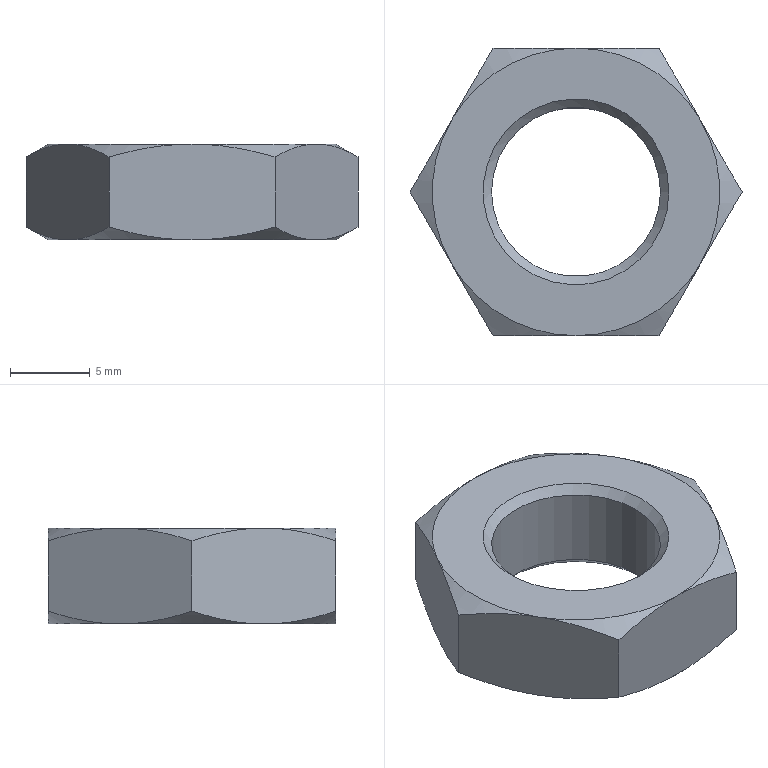Part | NX | features META 3, SKETCH 3, DATUM_CSYS 2, EXTRUDE 2, SWP104 2, CHAMFER 1, LINE 1, SYMBOLIC_THREAD 1, THREADS 1 | 1 solid | 23 faces | box 20.785 x 18 x 6 mm | volume 1134 mm3 | cone 14 | plane 8 | cylinder 1 | commonest cylinder face diameters 10.579 x1
STEP:
#1=CARTESIAN_POINT('',(5.819,0.,6.));
#2=VERTEX_POINT('',#1);
#3=CARTESIAN_POINT('',(0.,0.,6.));
#4=DIRECTION('',(0.,0.,1.));
#5=DIRECTION('',(1.,0.,0.));
#6=AXIS2_PLACEMENT_3D('',#3,#4,#5);
#7=CIRCLE('',#6,5.819);
#8=EDGE_CURVE('',#2,#2,#7,.F.);
#9=ORIENTED_EDGE('',*,*,#8,.T.);
#10=EDGE_LOOP('',(#9));
#11=FACE_BOUND('',#10,.T.);
#12=CARTESIAN_POINT('',(-7.794,4.5,6.));
#13=VERTEX_POINT('',#12);
#14=CARTESIAN_POINT('',(0.,9.,6.));
#15=VERTEX_POINT('',#14);
#16=CARTESIAN_POINT('',(0.,0.,6.));
#17=DIRECTION('',(0.,0.,-1.));
#18=DIRECTION('',(-1.,0.,0.));
#19=AXIS2_PLACEMENT_3D('',#16,#17,#18);
#20=CIRCLE('',#19,9.);
#21=EDGE_CURVE('',#13,#15,#20,.T.);
#22=ORIENTED_EDGE('',*,*,#21,.F.);
#23=CARTESIAN_POINT('',(-7.794,-4.5,6.));
#24=VERTEX_POINT('',#23);
#25=CARTESIAN_POINT('',(0.,0.,6.));
#26=DIRECTION('',(0.,0.,-1.));
#27=DIRECTION('',(-1.,0.,0.));
#28=AXIS2_PLACEMENT_3D('',#25,#26,#27);
#29=CIRCLE('',#28,9.);
#30=EDGE_CURVE('',#24,#13,#29,.T.);
#31=ORIENTED_EDGE('',*,*,#30,.F.);
#32=CARTESIAN_POINT('',(0.,-9.,6.));
#33=VERTEX_POINT('',#32);
#34=CARTESIAN_POINT('',(0.,0.,6.));
#35=DIRECTION('',(0.,0.,-1.));
#36=DIRECTION('',(-1.,0.,0.));
#37=AXIS2_PLACEMENT_3D('',#34,#35,#36);
#38=CIRCLE('',#37,9.);
#39=EDGE_CURVE('',#33,#24,#38,.T.);
#40=ORIENTED_EDGE('',*,*,#39,.F.);
#41=CARTESIAN_POINT('',(7.794,-4.5,6.));
#42=VERTEX_POINT('',#41);
#43=CARTESIAN_POINT('',(0.,0.,6.));
#44=DIRECTION('',(0.,0.,-1.));
#45=DIRECTION('',(-1.,0.,0.));
#46=AXIS2_PLACEMENT_3D('',#43,#44,#45);
#47=CIRCLE('',#46,9.);
#48=EDGE_CURVE('',#42,#33,#47,.T.);
#49=ORIENTED_EDGE('',*,*,#48,.F.);
#50=CARTESIAN_POINT('',(7.794,4.5,6.));
#51=VERTEX_POINT('',#50);
#52=CARTESIAN_POINT('',(0.,0.,6.));
#53=DIRECTION('',(0.,0.,-1.));
#54=DIRECTION('',(-1.,0.,0.));
#55=AXIS2_PLACEMENT_3D('',#52,#53,#54);
#56=CIRCLE('',#55,9.);
#57=EDGE_CURVE('',#51,#42,#56,.T.);
#58=ORIENTED_EDGE('',*,*,#57,.F.);
#59=CARTESIAN_POINT('',(0.,0.,6.));
#60=DIRECTION('',(0.,0.,-1.));
#61=DIRECTION('',(-1.,0.,0.));
#62=AXIS2_PLACEMENT_3D('',#59,#60,#61);
#63=CIRCLE('',#62,9.);
#64=EDGE_CURVE('',#15,#51,#63,.T.);
#65=ORIENTED_EDGE('',*,*,#64,.F.);
#66=EDGE_LOOP('',(#22,#31,#40,#49,#58,#65));
#67=FACE_BOUND('',#66,.T.);
#68=CARTESIAN_POINT('',(0.,18.,6.));
#69=DIRECTION('',(0.,0.,1.));
#70=DIRECTION('',(1.,0.,0.));
#71=AXIS2_PLACEMENT_3D('',#68,#69,#70);
#72=PLANE('',#71);
#73=ADVANCED_FACE('',(#11,#67),#72,.T.);
#74=CARTESIAN_POINT('',(5.819,0.,0.));
#75=VERTEX_POINT('',#74);
#76=CARTESIAN_POINT('',(0.,0.,0.));
#77=DIRECTION('',(0.,0.,1.));
#78=DIRECTION('',(1.,0.,0.));
#79=AXIS2_PLACEMENT_3D('',#76,#77,#78);
#80=CIRCLE('',#79,5.819);
#81=EDGE_CURVE('',#75,#75,#80,.T.);
#82=ORIENTED_EDGE('',*,*,#81,.T.);
#83=EDGE_LOOP('',(#82));
#84=FACE_BOUND('',#83,.T.);
#85=CARTESIAN_POINT('',(-7.794,-4.5,0.));
#86=VERTEX_POINT('',#85);
#87=CARTESIAN_POINT('',(-7.794,4.5,0.));
#88=VERTEX_POINT('',#87);
#89=CARTESIAN_POINT('',(0.,0.,0.));
#90=DIRECTION('',(0.,0.,-1.));
#91=DIRECTION('',(-1.,0.,0.));
#92=AXIS2_PLACEMENT_3D('',#89,#90,#91);
#93=CIRCLE('',#92,9.);
#94=EDGE_CURVE('',#86,#88,#93,.T.);
#95=ORIENTED_EDGE('',*,*,#94,.T.);
#96=CARTESIAN_POINT('',(0.,9.,0.));
#97=VERTEX_POINT('',#96);
#98=CARTESIAN_POINT('',(0.,0.,0.));
#99=DIRECTION('',(0.,0.,-1.));
#100=DIRECTION('',(-1.,0.,0.));
#101=AXIS2_PLACEMENT_3D('',#98,#99,#100);
#102=CIRCLE('',#101,9.);
#103=EDGE_CURVE('',#88,#97,#102,.T.);
#104=ORIENTED_EDGE('',*,*,#103,.T.);
#105=CARTESIAN_POINT('',(7.794,4.5,0.));
#106=VERTEX_POINT('',#105);
#107=CARTESIAN_POINT('',(0.,0.,0.));
#108=DIRECTION('',(0.,0.,-1.));
#109=DIRECTION('',(-1.,0.,0.));
#110=AXIS2_PLACEMENT_3D('',#107,#108,#109);
#111=CIRCLE('',#110,9.);
#112=EDGE_CURVE('',#97,#106,#111,.T.);
#113=ORIENTED_EDGE('',*,*,#112,.T.);
#114=CARTESIAN_POINT('',(7.794,-4.5,0.));
#115=VERTEX_POINT('',#114);
#116=CARTESIAN_POINT('',(0.,0.,0.));
#117=DIRECTION('',(0.,0.,-1.));
#118=DIRECTION('',(-1.,0.,0.));
#119=AXIS2_PLACEMENT_3D('',#116,#117,#118);
#120=CIRCLE('',#119,9.);
#121=EDGE_CURVE('',#106,#115,#120,.T.);
#122=ORIENTED_EDGE('',*,*,#121,.T.);
#123=CARTESIAN_POINT('',(0.,-9.,0.));
#124=VERTEX_POINT('',#123);
#125=CARTESIAN_POINT('',(0.,0.,0.));
#126=DIRECTION('',(0.,0.,-1.));
#127=DIRECTION('',(-1.,0.,0.));
#128=AXIS2_PLACEMENT_3D('',#125,#126,#127);
#129=CIRCLE('',#128,9.);
#130=EDGE_CURVE('',#115,#124,#129,.T.);
#131=ORIENTED_EDGE('',*,*,#130,.T.);
#132=CARTESIAN_POINT('',(0.,0.,0.));
#133=DIRECTION('',(0.,0.,-1.));
#134=DIRECTION('',(-1.,0.,0.));
#135=AXIS2_PLACEMENT_3D('',#132,#133,#134);
#136=CIRCLE('',#135,9.);
#137=EDGE_CURVE('',#124,#86,#136,.T.);
#138=ORIENTED_EDGE('',*,*,#137,.T.);
#139=EDGE_LOOP('',(#95,#104,#113,#122,#131,#138));
#140=FACE_BOUND('',#139,.T.);
#141=CARTESIAN_POINT('',(0.,18.,0.));
#142=DIRECTION('',(0.,0.,1.));
#143=DIRECTION('',(1.,0.,0.));
#144=AXIS2_PLACEMENT_3D('',#141,#142,#143);
#145=PLANE('',#144);
#146=ADVANCED_FACE('',(#84,#140),#145,.F.);
#147=CARTESIAN_POINT('',(10.392,0.,5.196));
#148=VERTEX_POINT('',#147);
#149=CARTESIAN_POINT('',(10.392,0.,0.8038));
#150=VERTEX_POINT('',#149);
#151=CARTESIAN_POINT('',(10.392,0.,6.));
#152=DIRECTION('',(0.,0.,-1.));
#153=VECTOR('',#152,1000.);
#154=LINE('',#151,#153);
#155=EDGE_CURVE('',#148,#150,#154,.T.);
#156=ORIENTED_EDGE('',*,*,#155,.T.);
#157=CARTESIAN_POINT('',(10.392,0.,0.8038));
#158=CARTESIAN_POINT('',(9.542,1.472,0.3131));
#159=CARTESIAN_POINT('',(8.679,2.967,0.));
#160=CARTESIAN_POINT('',(7.794,4.5,0.));
#161=B_SPLINE_CURVE_WITH_KNOTS('',3,(#157,#158,#159,#160),.UNSPECIFIED.,.F.,.F.,(4,4),(0.000000238,0.005258),.UNSPECIFIED.);
#162=EDGE_CURVE('',#150,#106,#161,.T.);
#163=ORIENTED_EDGE('',*,*,#162,.T.);
#164=CARTESIAN_POINT('',(5.196,9.,0.8038));
#165=VERTEX_POINT('',#164);
#166=CARTESIAN_POINT('',(7.794,4.5,0.));
#167=CARTESIAN_POINT('',(6.912,6.028,0.));
#168=CARTESIAN_POINT('',(6.044,7.531,0.3143));
#169=CARTESIAN_POINT('',(5.196,9.,0.8038));
#170=B_SPLINE_CURVE_WITH_KNOTS('',3,(#166,#167,#168,#169),.UNSPECIFIED.,.F.,.F.,(4,4),(0.005258,0.0105),.UNSPECIFIED.);
#171=EDGE_CURVE('',#106,#165,#170,.T.);
#172=ORIENTED_EDGE('',*,*,#171,.T.);
#173=CARTESIAN_POINT('',(5.196,9.,5.196));
#174=VERTEX_POINT('',#173);
#175=CARTESIAN_POINT('',(5.196,9.,6.));
#176=DIRECTION('',(0.,0.,-1.));
#177=VECTOR('',#176,1000.);
#178=LINE('',#175,#177);
#179=EDGE_CURVE('',#174,#165,#178,.T.);
#180=ORIENTED_EDGE('',*,*,#179,.F.);
#181=CARTESIAN_POINT('',(5.196,9.,5.196));
#182=CARTESIAN_POINT('',(6.046,7.528,5.687));
#183=CARTESIAN_POINT('',(6.909,6.033,6.));
#184=CARTESIAN_POINT('',(7.794,4.5,6.));
#185=B_SPLINE_CURVE_WITH_KNOTS('',3,(#181,#182,#183,#184),.UNSPECIFIED.,.F.,.F.,(4,4),(0.000000238,0.005258),.UNSPECIFIED.);
#186=EDGE_CURVE('',#174,#51,#185,.T.);
#187=ORIENTED_EDGE('',*,*,#186,.T.);
#188=CARTESIAN_POINT('',(7.794,4.5,6.));
#189=CARTESIAN_POINT('',(8.676,2.972,6.));
#190=CARTESIAN_POINT('',(9.544,1.469,5.686));
#191=CARTESIAN_POINT('',(10.392,0.,5.196));
#192=B_SPLINE_CURVE_WITH_KNOTS('',3,(#188,#189,#190,#191),.UNSPECIFIED.,.F.,.F.,(4,4),(0.005258,0.0105),.UNSPECIFIED.);
#193=EDGE_CURVE('',#51,#148,#192,.T.);
#194=ORIENTED_EDGE('',*,*,#193,.T.);
#195=EDGE_LOOP('',(#156,#163,#172,#180,#187,#194));
#196=FACE_BOUND('',#195,.T.);
#197=CARTESIAN_POINT('',(5.196,9.,6.));
#198=DIRECTION('',(0.866,0.5,0.));
#199=DIRECTION('',(-0.5,0.866,0.));
#200=AXIS2_PLACEMENT_3D('',#197,#198,#199);
#201=PLANE('',#200);
#202=ADVANCED_FACE('',(#196),#201,.T.);
#203=CARTESIAN_POINT('',(5.196,-9.,5.196));
#204=VERTEX_POINT('',#203);
#205=CARTESIAN_POINT('',(5.196,-9.,0.8038));
#206=VERTEX_POINT('',#205);
#207=CARTESIAN_POINT('',(5.196,-9.,6.));
#208=DIRECTION('',(0.,0.,-1.));
#209=VECTOR('',#208,1000.);
#210=LINE('',#207,#209);
#211=EDGE_CURVE('',#204,#206,#210,.T.);
#212=ORIENTED_EDGE('',*,*,#211,.T.);
#213=CARTESIAN_POINT('',(5.196,-9.,0.8038));
#214=CARTESIAN_POINT('',(6.046,-7.528,0.3131));
#215=CARTESIAN_POINT('',(6.909,-6.033,0.));
#216=CARTESIAN_POINT('',(7.794,-4.5,0.));
#217=B_SPLINE_CURVE_WITH_KNOTS('',3,(#213,#214,#215,#216),.UNSPECIFIED.,.F.,.F.,(4,4),(0.000000238,0.005258),.UNSPECIFIED.);
#218=EDGE_CURVE('',#206,#115,#217,.T.);
#219=ORIENTED_EDGE('',*,*,#218,.T.);
#220=CARTESIAN_POINT('',(7.794,-4.5,0.));
#221=CARTESIAN_POINT('',(8.676,-2.972,0.));
#222=CARTESIAN_POINT('',(9.544,-1.469,0.3143));
#223=CARTESIAN_POINT('',(10.392,0.,0.8038));
#224=B_SPLINE_CURVE_WITH_KNOTS('',3,(#220,#221,#222,#223),.UNSPECIFIED.,.F.,.F.,(4,4),(0.005258,0.0105),.UNSPECIFIED.);
#225=EDGE_CURVE('',#115,#150,#224,.T.);
#226=ORIENTED_EDGE('',*,*,#225,.T.);
#227=ORIENTED_EDGE('',*,*,#155,.F.);
#228=CARTESIAN_POINT('',(10.392,0.,5.196));
#229=CARTESIAN_POINT('',(9.542,-1.472,5.687));
#230=CARTESIAN_POINT('',(8.679,-2.967,6.));
#231=CARTESIAN_POINT('',(7.794,-4.5,6.));
#232=B_SPLINE_CURVE_WITH_KNOTS('',3,(#228,#229,#230,#231),.UNSPECIFIED.,.F.,.F.,(4,4),(0.000000238,0.005258),.UNSPECIFIED.);
#233=EDGE_CURVE('',#148,#42,#232,.T.);
#234=ORIENTED_EDGE('',*,*,#233,.T.);
#235=CARTESIAN_POINT('',(7.794,-4.5,6.));
#236=CARTESIAN_POINT('',(6.912,-6.028,6.));
#237=CARTESIAN_POINT('',(6.044,-7.531,5.686));
#238=CARTESIAN_POINT('',(5.196,-9.,5.196));
#239=B_SPLINE_CURVE_WITH_KNOTS('',3,(#235,#236,#237,#238),.UNSPECIFIED.,.F.,.F.,(4,4),(0.005258,0.0105),.UNSPECIFIED.);
#240=EDGE_CURVE('',#42,#204,#239,.T.);
#241=ORIENTED_EDGE('',*,*,#240,.T.);
#242=EDGE_LOOP('',(#212,#219,#226,#227,#234,#241));
#243=FACE_BOUND('',#242,.T.);
#244=CARTESIAN_POINT('',(10.392,0.,6.));
#245=DIRECTION('',(0.866,-0.5,0.));
#246=DIRECTION('',(0.5,0.866,0.));
#247=AXIS2_PLACEMENT_3D('',#244,#245,#246);
#248=PLANE('',#247);
#249=ADVANCED_FACE('',(#243),#248,.T.);
#250=CARTESIAN_POINT('',(-5.196,-9.,5.196));
#251=VERTEX_POINT('',#250);
#252=CARTESIAN_POINT('',(-5.196,-9.,0.8038));
#253=VERTEX_POINT('',#252);
#254=CARTESIAN_POINT('',(-5.196,-9.,6.));
#255=DIRECTION('',(0.,0.,-1.));
#256=VECTOR('',#255,1000.);
#257=LINE('',#254,#256);
#258=EDGE_CURVE('',#251,#253,#257,.T.);
#259=ORIENTED_EDGE('',*,*,#258,.T.);
#260=CARTESIAN_POINT('',(-5.196,-9.,0.8038));
#261=CARTESIAN_POINT('',(-3.506,-9.,0.3159));
#262=CARTESIAN_POINT('',(-1.756,-9.,0.));
#263=CARTESIAN_POINT('',(0.,-9.,0.));
#264=B_SPLINE_CURVE_WITH_KNOTS('',3,(#260,#261,#262,#263),.UNSPECIFIED.,.F.,.F.,(4,4),(0.009271,0.01453),.UNSPECIFIED.);
#265=EDGE_CURVE('',#253,#124,#264,.T.);
#266=ORIENTED_EDGE('',*,*,#265,.T.);
#267=CARTESIAN_POINT('',(0.,-9.,0.));
#268=CARTESIAN_POINT('',(1.757,-9.,0.));
#269=CARTESIAN_POINT('',(3.516,-9.,0.3188));
#270=CARTESIAN_POINT('',(5.196,-9.,0.8038));
#271=B_SPLINE_CURVE_WITH_KNOTS('',3,(#267,#268,#269,#270),.UNSPECIFIED.,.F.,.F.,(4,4),(0.01453,0.01979),.UNSPECIFIED.);
#272=EDGE_CURVE('',#124,#206,#271,.T.);
#273=ORIENTED_EDGE('',*,*,#272,.T.);
#274=ORIENTED_EDGE('',*,*,#211,.F.);
#275=CARTESIAN_POINT('',(0.,-9.,6.));
#276=CARTESIAN_POINT('',(1.757,-9.,6.));
#277=CARTESIAN_POINT('',(3.516,-9.,5.681));
#278=CARTESIAN_POINT('',(5.196,-9.,5.196));
#279=B_SPLINE_CURVE_WITH_KNOTS('',3,(#275,#276,#277,#278),.UNSPECIFIED.,.F.,.F.,(4,4),(0.01453,0.01979),.UNSPECIFIED.);
#280=EDGE_CURVE('',#204,#33,#279,.F.);
#281=ORIENTED_EDGE('',*,*,#280,.T.);
#282=CARTESIAN_POINT('',(-5.196,-9.,5.196));
#283=CARTESIAN_POINT('',(-3.506,-9.,5.684));
#284=CARTESIAN_POINT('',(-1.756,-9.,6.));
#285=CARTESIAN_POINT('',(0.,-9.,6.));
#286=B_SPLINE_CURVE_WITH_KNOTS('',3,(#282,#283,#284,#285),.UNSPECIFIED.,.F.,.F.,(4,4),(0.009271,0.01453),.UNSPECIFIED.);
#287=EDGE_CURVE('',#33,#251,#286,.F.);
#288=ORIENTED_EDGE('',*,*,#287,.T.);
#289=EDGE_LOOP('',(#259,#266,#273,#274,#281,#288));
#290=FACE_BOUND('',#289,.T.);
#291=CARTESIAN_POINT('',(5.196,-9.,6.));
#292=DIRECTION('',(0.,-1.,0.));
#293=DIRECTION('',(0.,0.,-1.));
#294=AXIS2_PLACEMENT_3D('',#291,#292,#293);
#295=PLANE('',#294);
#296=ADVANCED_FACE('',(#290),#295,.T.);
#297=CARTESIAN_POINT('',(-10.392,0.,5.196));
#298=VERTEX_POINT('',#297);
#299=CARTESIAN_POINT('',(-10.392,0.,0.8038));
#300=VERTEX_POINT('',#299);
#301=CARTESIAN_POINT('',(-10.392,0.,6.));
#302=DIRECTION('',(0.,0.,-1.));
#303=VECTOR('',#302,1000.);
#304=LINE('',#301,#303);
#305=EDGE_CURVE('',#298,#300,#304,.T.);
#306=ORIENTED_EDGE('',*,*,#305,.T.);
#307=CARTESIAN_POINT('',(-10.392,0.,0.8038));
#308=CARTESIAN_POINT('',(-9.542,-1.472,0.3131));
#309=CARTESIAN_POINT('',(-8.679,-2.967,0.));
#310=CARTESIAN_POINT('',(-7.794,-4.5,0.));
#311=B_SPLINE_CURVE_WITH_KNOTS('',3,(#307,#308,#309,#310),.UNSPECIFIED.,.F.,.F.,(4,4),(0.000000238,0.005258),.UNSPECIFIED.);
#312=EDGE_CURVE('',#300,#86,#311,.T.);
#313=ORIENTED_EDGE('',*,*,#312,.T.);
#314=CARTESIAN_POINT('',(-7.794,-4.5,0.));
#315=CARTESIAN_POINT('',(-6.912,-6.028,0.));
#316=CARTESIAN_POINT('',(-6.044,-7.531,0.3143));
#317=CARTESIAN_POINT('',(-5.196,-9.,0.8038));
#318=B_SPLINE_CURVE_WITH_KNOTS('',3,(#314,#315,#316,#317),.UNSPECIFIED.,.F.,.F.,(4,4),(0.005258,0.0105),.UNSPECIFIED.);
#319=EDGE_CURVE('',#86,#253,#318,.T.);
#320=ORIENTED_EDGE('',*,*,#319,.T.);
#321=ORIENTED_EDGE('',*,*,#258,.F.);
#322=CARTESIAN_POINT('',(-5.196,-9.,5.196));
#323=CARTESIAN_POINT('',(-6.046,-7.528,5.687));
#324=CARTESIAN_POINT('',(-6.909,-6.033,6.));
#325=CARTESIAN_POINT('',(-7.794,-4.5,6.));
#326=B_SPLINE_CURVE_WITH_KNOTS('',3,(#322,#323,#324,#325),.UNSPECIFIED.,.F.,.F.,(4,4),(0.000000238,0.005258),.UNSPECIFIED.);
#327=EDGE_CURVE('',#251,#24,#326,.T.);
#328=ORIENTED_EDGE('',*,*,#327,.T.);
#329=CARTESIAN_POINT('',(-7.794,-4.5,6.));
#330=CARTESIAN_POINT('',(-8.676,-2.972,6.));
#331=CARTESIAN_POINT('',(-9.544,-1.469,5.686));
#332=CARTESIAN_POINT('',(-10.392,0.,5.196));
#333=B_SPLINE_CURVE_WITH_KNOTS('',3,(#329,#330,#331,#332),.UNSPECIFIED.,.F.,.F.,(4,4),(0.005258,0.0105),.UNSPECIFIED.);
#334=EDGE_CURVE('',#24,#298,#333,.T.);
#335=ORIENTED_EDGE('',*,*,#334,.T.);
#336=EDGE_LOOP('',(#306,#313,#320,#321,#328,#335));
#337=FACE_BOUND('',#336,.T.);
#338=CARTESIAN_POINT('',(-5.196,-9.,6.));
#339=DIRECTION('',(-0.866,-0.5,0.));
#340=DIRECTION('',(0.5,-0.866,0.));
#341=AXIS2_PLACEMENT_3D('',#338,#339,#340);
#342=PLANE('',#341);
#343=ADVANCED_FACE('',(#337),#342,.T.);
#344=CARTESIAN_POINT('',(-5.196,9.,5.196));
#345=VERTEX_POINT('',#344);
#346=CARTESIAN_POINT('',(-5.196,9.,0.8038));
#347=VERTEX_POINT('',#346);
#348=CARTESIAN_POINT('',(-5.196,9.,6.));
#349=DIRECTION('',(0.,0.,-1.));
#350=VECTOR('',#349,1000.);
#351=LINE('',#348,#350);
#352=EDGE_CURVE('',#345,#347,#351,.T.);
#353=ORIENTED_EDGE('',*,*,#352,.T.);
#354=CARTESIAN_POINT('',(-5.196,9.,0.8038));
#355=CARTESIAN_POINT('',(-6.046,7.528,0.3131));
#356=CARTESIAN_POINT('',(-6.909,6.033,0.));
#357=CARTESIAN_POINT('',(-7.794,4.5,0.));
#358=B_SPLINE_CURVE_WITH_KNOTS('',3,(#354,#355,#356,#357),.UNSPECIFIED.,.F.,.F.,(4,4),(0.000000238,0.005258),.UNSPECIFIED.);
#359=EDGE_CURVE('',#347,#88,#358,.T.);
#360=ORIENTED_EDGE('',*,*,#359,.T.);
#361=CARTESIAN_POINT('',(-7.794,4.5,0.));
#362=CARTESIAN_POINT('',(-8.676,2.972,0.));
#363=CARTESIAN_POINT('',(-9.544,1.469,0.3143));
#364=CARTESIAN_POINT('',(-10.392,0.,0.8038));
#365=B_SPLINE_CURVE_WITH_KNOTS('',3,(#361,#362,#363,#364),.UNSPECIFIED.,.F.,.F.,(4,4),(0.005258,0.0105),.UNSPECIFIED.);
#366=EDGE_CURVE('',#88,#300,#365,.T.);
#367=ORIENTED_EDGE('',*,*,#366,.T.);
#368=ORIENTED_EDGE('',*,*,#305,.F.);
#369=CARTESIAN_POINT('',(-10.392,0.,5.196));
#370=CARTESIAN_POINT('',(-9.542,1.472,5.687));
#371=CARTESIAN_POINT('',(-8.679,2.967,6.));
#372=CARTESIAN_POINT('',(-7.794,4.5,6.));
#373=B_SPLINE_CURVE_WITH_KNOTS('',3,(#369,#370,#371,#372),.UNSPECIFIED.,.F.,.F.,(4,4),(0.000000238,0.005258),.UNSPECIFIED.);
#374=EDGE_CURVE('',#298,#13,#373,.T.);
#375=ORIENTED_EDGE('',*,*,#374,.T.);
#376=CARTESIAN_POINT('',(-7.794,4.5,6.));
#377=CARTESIAN_POINT('',(-6.912,6.028,6.));
#378=CARTESIAN_POINT('',(-6.044,7.531,5.686));
#379=CARTESIAN_POINT('',(-5.196,9.,5.196));
#380=B_SPLINE_CURVE_WITH_KNOTS('',3,(#376,#377,#378,#379),.UNSPECIFIED.,.F.,.F.,(4,4),(0.005258,0.0105),.UNSPECIFIED.);
#381=EDGE_CURVE('',#13,#345,#380,.T.);
#382=ORIENTED_EDGE('',*,*,#381,.T.);
#383=EDGE_LOOP('',(#353,#360,#367,#368,#375,#382));
#384=FACE_BOUND('',#383,.T.);
#385=CARTESIAN_POINT('',(-10.392,0.,6.));
#386=DIRECTION('',(-0.866,0.5,0.));
#387=DIRECTION('',(-0.5,-0.866,0.));
#388=AXIS2_PLACEMENT_3D('',#385,#386,#387);
#389=PLANE('',#388);
#390=ADVANCED_FACE('',(#384),#389,.T.);
#391=ORIENTED_EDGE('',*,*,#179,.T.);
#392=CARTESIAN_POINT('',(0.,9.,0.));
#393=CARTESIAN_POINT('',(1.757,9.,0.));
#394=CARTESIAN_POINT('',(3.516,9.,0.3188));
#395=CARTESIAN_POINT('',(5.196,9.,0.8038));
#396=B_SPLINE_CURVE_WITH_KNOTS('',3,(#392,#393,#394,#395),.UNSPECIFIED.,.F.,.F.,(4,4),(0.01453,0.01979),.UNSPECIFIED.);
#397=EDGE_CURVE('',#165,#97,#396,.F.);
#398=ORIENTED_EDGE('',*,*,#397,.T.);
#399=CARTESIAN_POINT('',(-5.196,9.,0.8038));
#400=CARTESIAN_POINT('',(-3.506,9.,0.3159));
#401=CARTESIAN_POINT('',(-1.756,9.,0.));
#402=CARTESIAN_POINT('',(0.,9.,0.));
#403=B_SPLINE_CURVE_WITH_KNOTS('',3,(#399,#400,#401,#402),.UNSPECIFIED.,.F.,.F.,(4,4),(0.009271,0.01453),.UNSPECIFIED.);
#404=EDGE_CURVE('',#97,#347,#403,.F.);
#405=ORIENTED_EDGE('',*,*,#404,.T.);
#406=ORIENTED_EDGE('',*,*,#352,.F.);
#407=CARTESIAN_POINT('',(-5.196,9.,5.196));
#408=CARTESIAN_POINT('',(-3.506,9.,5.684));
#409=CARTESIAN_POINT('',(-1.756,9.,6.));
#410=CARTESIAN_POINT('',(0.,9.,6.));
#411=B_SPLINE_CURVE_WITH_KNOTS('',3,(#407,#408,#409,#410),.UNSPECIFIED.,.F.,.F.,(4,4),(0.009271,0.01453),.UNSPECIFIED.);
#412=EDGE_CURVE('',#345,#15,#411,.T.);
#413=ORIENTED_EDGE('',*,*,#412,.T.);
#414=CARTESIAN_POINT('',(0.,9.,6.));
#415=CARTESIAN_POINT('',(1.757,9.,6.));
#416=CARTESIAN_POINT('',(3.516,9.,5.681));
#417=CARTESIAN_POINT('',(5.196,9.,5.196));
#418=B_SPLINE_CURVE_WITH_KNOTS('',3,(#414,#415,#416,#417),.UNSPECIFIED.,.F.,.F.,(4,4),(0.01453,0.01979),.UNSPECIFIED.);
#419=EDGE_CURVE('',#15,#174,#418,.T.);
#420=ORIENTED_EDGE('',*,*,#419,.T.);
#421=EDGE_LOOP('',(#391,#398,#405,#406,#413,#420));
#422=FACE_BOUND('',#421,.T.);
#423=CARTESIAN_POINT('',(-5.196,9.,6.));
#424=DIRECTION('',(0.,1.,0.));
#425=DIRECTION('',(0.,0.,1.));
#426=AXIS2_PLACEMENT_3D('',#423,#424,#425);
#427=PLANE('',#426);
#428=ADVANCED_FACE('',(#422),#427,.T.);
#429=ORIENTED_EDGE('',*,*,#419,.F.);
#430=ORIENTED_EDGE('',*,*,#64,.T.);
#431=ORIENTED_EDGE('',*,*,#186,.F.);
#432=EDGE_LOOP('',(#429,#430,#431));
#433=FACE_BOUND('',#432,.T.);
#434=CARTESIAN_POINT('',(0.,0.,5.196));
#435=DIRECTION('',(0.,0.,-1.));
#436=DIRECTION('',(-1.,0.,0.));
#437=AXIS2_PLACEMENT_3D('',#434,#435,#436);
#438=CONICAL_SURFACE('',#437,10.392,1.047);
#439=ADVANCED_FACE('',(#433),#438,.T.);
#440=ORIENTED_EDGE('',*,*,#21,.T.);
#441=ORIENTED_EDGE('',*,*,#412,.F.);
#442=ORIENTED_EDGE('',*,*,#381,.F.);
#443=EDGE_LOOP('',(#440,#441,#442));
#444=FACE_BOUND('',#443,.T.);
#445=CARTESIAN_POINT('',(0.,0.,5.196));
#446=DIRECTION('',(0.,0.,-1.));
#447=DIRECTION('',(-1.,0.,0.));
#448=AXIS2_PLACEMENT_3D('',#445,#446,#447);
#449=CONICAL_SURFACE('',#448,10.392,1.047);
#450=ADVANCED_FACE('',(#444),#449,.T.);
#451=ORIENTED_EDGE('',*,*,#30,.T.);
#452=ORIENTED_EDGE('',*,*,#374,.F.);
#453=ORIENTED_EDGE('',*,*,#334,.F.);
#454=EDGE_LOOP('',(#451,#452,#453));
#455=FACE_BOUND('',#454,.T.);
#456=CARTESIAN_POINT('',(0.,0.,5.196));
#457=DIRECTION('',(0.,0.,-1.));
#458=DIRECTION('',(-1.,0.,0.));
#459=AXIS2_PLACEMENT_3D('',#456,#457,#458);
#460=CONICAL_SURFACE('',#459,10.392,1.047);
#461=ADVANCED_FACE('',(#455),#460,.T.);
#462=ORIENTED_EDGE('',*,*,#39,.T.);
#463=ORIENTED_EDGE('',*,*,#327,.F.);
#464=ORIENTED_EDGE('',*,*,#287,.F.);
#465=EDGE_LOOP('',(#462,#463,#464));
#466=FACE_BOUND('',#465,.T.);
#467=CARTESIAN_POINT('',(0.,0.,5.196));
#468=DIRECTION('',(0.,0.,-1.));
#469=DIRECTION('',(-1.,0.,0.));
#470=AXIS2_PLACEMENT_3D('',#467,#468,#469);
#471=CONICAL_SURFACE('',#470,10.392,1.047);
#472=ADVANCED_FACE('',(#466),#471,.T.);
#473=ORIENTED_EDGE('',*,*,#48,.T.);
#474=ORIENTED_EDGE('',*,*,#280,.F.);
#475=ORIENTED_EDGE('',*,*,#240,.F.);
#476=EDGE_LOOP('',(#473,#474,#475));
#477=FACE_BOUND('',#476,.T.);
#478=CARTESIAN_POINT('',(0.,0.,5.196));
#479=DIRECTION('',(0.,0.,-1.));
#480=DIRECTION('',(-1.,0.,0.));
#481=AXIS2_PLACEMENT_3D('',#478,#479,#480);
#482=CONICAL_SURFACE('',#481,10.392,1.047);
#483=ADVANCED_FACE('',(#477),#482,.T.);
#484=ORIENTED_EDGE('',*,*,#57,.T.);
#485=ORIENTED_EDGE('',*,*,#233,.F.);
#486=ORIENTED_EDGE('',*,*,#193,.F.);
#487=EDGE_LOOP('',(#484,#485,#486));
#488=FACE_BOUND('',#487,.T.);
#489=CARTESIAN_POINT('',(0.,0.,5.196));
#490=DIRECTION('',(0.,0.,-1.));
#491=DIRECTION('',(-1.,0.,0.));
#492=AXIS2_PLACEMENT_3D('',#489,#490,#491);
#493=CONICAL_SURFACE('',#492,10.392,1.047);
#494=ADVANCED_FACE('',(#488),#493,.T.);
#495=ORIENTED_EDGE('',*,*,#404,.F.);
#496=ORIENTED_EDGE('',*,*,#103,.F.);
#497=ORIENTED_EDGE('',*,*,#359,.F.);
#498=EDGE_LOOP('',(#495,#496,#497));
#499=FACE_BOUND('',#498,.T.);
#500=CARTESIAN_POINT('',(0.,0.,0.));
#501=DIRECTION('',(0.,0.,1.));
#502=DIRECTION('',(1.,0.,0.));
#503=AXIS2_PLACEMENT_3D('',#500,#501,#502);
#504=CONICAL_SURFACE('',#503,9.,1.047);
#505=ADVANCED_FACE('',(#499),#504,.T.);
#506=ORIENTED_EDGE('',*,*,#112,.F.);
#507=ORIENTED_EDGE('',*,*,#397,.F.);
#508=ORIENTED_EDGE('',*,*,#171,.F.);
#509=EDGE_LOOP('',(#506,#507,#508));
#510=FACE_BOUND('',#509,.T.);
#511=CARTESIAN_POINT('',(0.,0.,0.));
#512=DIRECTION('',(0.,0.,1.));
#513=DIRECTION('',(1.,0.,0.));
#514=AXIS2_PLACEMENT_3D('',#511,#512,#513);
#515=CONICAL_SURFACE('',#514,9.,1.047);
#516=ADVANCED_FACE('',(#510),#515,.T.);
#517=ORIENTED_EDGE('',*,*,#366,.F.);
#518=ORIENTED_EDGE('',*,*,#94,.F.);
#519=ORIENTED_EDGE('',*,*,#312,.F.);
#520=EDGE_LOOP('',(#517,#518,#519));
#521=FACE_BOUND('',#520,.T.);
#522=CARTESIAN_POINT('',(0.,0.,0.));
#523=DIRECTION('',(0.,0.,1.));
#524=DIRECTION('',(1.,0.,0.));
#525=AXIS2_PLACEMENT_3D('',#522,#523,#524);
#526=CONICAL_SURFACE('',#525,9.,1.047);
#527=ADVANCED_FACE('',(#521),#526,.T.);
#528=ORIENTED_EDGE('',*,*,#319,.F.);
#529=ORIENTED_EDGE('',*,*,#137,.F.);
#530=ORIENTED_EDGE('',*,*,#265,.F.);
#531=EDGE_LOOP('',(#528,#529,#530));
#532=FACE_BOUND('',#531,.T.);
#533=CARTESIAN_POINT('',(0.,0.,0.));
#534=DIRECTION('',(0.,0.,1.));
#535=DIRECTION('',(1.,0.,0.));
#536=AXIS2_PLACEMENT_3D('',#533,#534,#535);
#537=CONICAL_SURFACE('',#536,9.,1.047);
#538=ADVANCED_FACE('',(#532),#537,.T.);
#539=ORIENTED_EDGE('',*,*,#130,.F.);
#540=ORIENTED_EDGE('',*,*,#218,.F.);
#541=ORIENTED_EDGE('',*,*,#272,.F.);
#542=EDGE_LOOP('',(#539,#540,#541));
#543=FACE_BOUND('',#542,.T.);
#544=CARTESIAN_POINT('',(0.,0.,0.));
#545=DIRECTION('',(0.,0.,1.));
#546=DIRECTION('',(1.,0.,0.));
#547=AXIS2_PLACEMENT_3D('',#544,#545,#546);
#548=CONICAL_SURFACE('',#547,9.,1.047);
#549=ADVANCED_FACE('',(#543),#548,.T.);
#550=ORIENTED_EDGE('',*,*,#121,.F.);
#551=ORIENTED_EDGE('',*,*,#162,.F.);
#552=ORIENTED_EDGE('',*,*,#225,.F.);
#553=EDGE_LOOP('',(#550,#551,#552));
#554=FACE_BOUND('',#553,.T.);
#555=CARTESIAN_POINT('',(0.,0.,0.));
#556=DIRECTION('',(0.,0.,1.));
#557=DIRECTION('',(1.,0.,0.));
#558=AXIS2_PLACEMENT_3D('',#555,#556,#557);
#559=CONICAL_SURFACE('',#558,9.,1.047);
#560=ADVANCED_FACE('',(#554),#559,.T.);
#561=CARTESIAN_POINT('',(5.29,0.,0.529));
#562=VERTEX_POINT('',#561);
#563=CARTESIAN_POINT('',(0.,0.,0.529));
#564=DIRECTION('',(0.,0.,1.));
#565=DIRECTION('',(1.,0.,0.));
#566=AXIS2_PLACEMENT_3D('',#563,#564,#565);
#567=CIRCLE('',#566,5.29);
#568=EDGE_CURVE('',#562,#562,#567,.F.);
#569=ORIENTED_EDGE('',*,*,#568,.T.);
#570=EDGE_LOOP('',(#569));
#571=FACE_BOUND('',#570,.T.);
#572=CARTESIAN_POINT('',(5.29,0.,5.471));
#573=VERTEX_POINT('',#572);
#574=CARTESIAN_POINT('',(0.,0.,5.471));
#575=DIRECTION('',(0.,0.,1.));
#576=DIRECTION('',(1.,0.,0.));
#577=AXIS2_PLACEMENT_3D('',#574,#575,#576);
#578=CIRCLE('',#577,5.29);
#579=EDGE_CURVE('',#573,#573,#578,.T.);
#580=ORIENTED_EDGE('',*,*,#579,.T.);
#581=EDGE_LOOP('',(#580));
#582=FACE_BOUND('',#581,.T.);
#583=CARTESIAN_POINT('',(0.,0.,6.));
#584=DIRECTION('',(0.,0.,-1.));
#585=DIRECTION('',(-1.,0.,0.));
#586=AXIS2_PLACEMENT_3D('',#583,#584,#585);
#587=CYLINDRICAL_SURFACE('',#586,5.29);
#588=ADVANCED_FACE('',(#571,#582),#587,.F.);
#589=ORIENTED_EDGE('',*,*,#81,.F.);
#590=EDGE_LOOP('',(#589));
#591=FACE_BOUND('',#590,.T.);
#592=ORIENTED_EDGE('',*,*,#568,.F.);
#593=EDGE_LOOP('',(#592));
#594=FACE_BOUND('',#593,.T.);
#595=CARTESIAN_POINT('',(0.,0.,0.529));
#596=DIRECTION('',(0.,0.,-1.));
#597=DIRECTION('',(-1.,0.,0.));
#598=AXIS2_PLACEMENT_3D('',#595,#596,#597);
#599=CONICAL_SURFACE('',#598,5.29,0.7854);
#600=ADVANCED_FACE('',(#591,#594),#599,.F.);
#601=ORIENTED_EDGE('',*,*,#579,.F.);
#602=EDGE_LOOP('',(#601));
#603=FACE_BOUND('',#602,.T.);
#604=ORIENTED_EDGE('',*,*,#8,.F.);
#605=EDGE_LOOP('',(#604));
#606=FACE_BOUND('',#605,.T.);
#607=CARTESIAN_POINT('',(0.,0.,6.));
#608=DIRECTION('',(0.,0.,1.));
#609=DIRECTION('',(1.,0.,0.));
#610=AXIS2_PLACEMENT_3D('',#607,#608,#609);
#611=CONICAL_SURFACE('',#610,5.819,0.7854);
#612=ADVANCED_FACE('',(#603,#606),#611,.F.);
#613=CLOSED_SHELL('',(#73,#146,#202,#249,#296,#343,#390,#428,#439,#450,#461,#472,#483,#494,#505,#516,#527,#538,#549,#560,#588,#600,#612));
#614=MANIFOLD_SOLID_BREP('',#613);
#615=(LENGTH_UNIT()NAMED_UNIT(*)SI_UNIT(.MILLI.,.METRE.));
#616=UNCERTAINTY_MEASURE_WITH_UNIT(LENGTH_MEASURE(0.0508),#615,'','');
#617=(NAMED_UNIT(*)PLANE_ANGLE_UNIT()SI_UNIT($,.RADIAN.));
#618=(NAMED_UNIT(*)SI_UNIT($,.STERADIAN.)SOLID_ANGLE_UNIT());
#619=(GEOMETRIC_REPRESENTATION_CONTEXT(3)GLOBAL_UNCERTAINTY_ASSIGNED_CONTEXT((#616))GLOBAL_UNIT_ASSIGNED_CONTEXT((#615,#617,#618))REPRESENTATION_CONTEXT('',''));
#620=ADVANCED_BREP_SHAPE_REPRESENTATION('',(#614),#619);